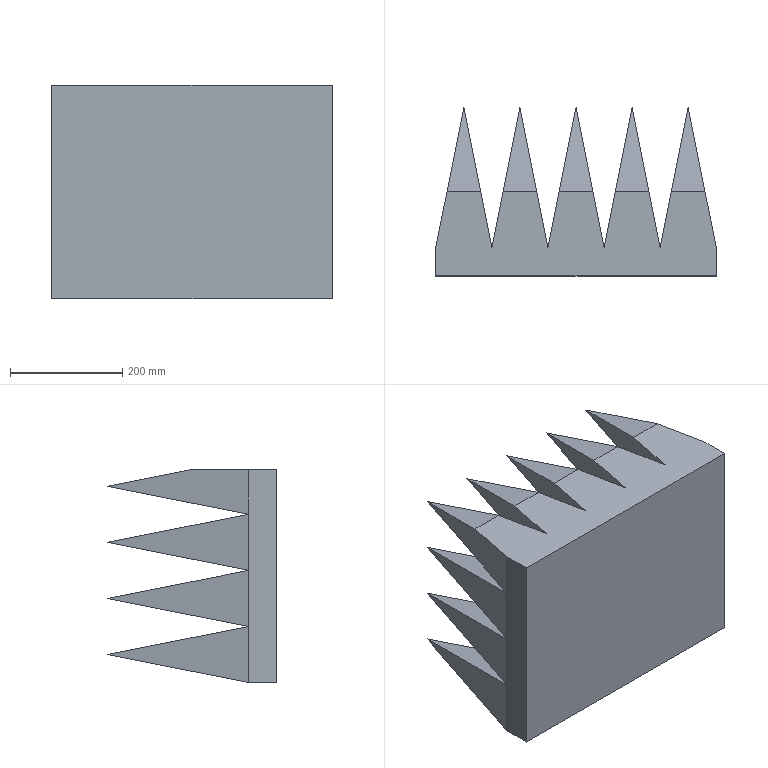Part | SolidWorks | features LPattern 2, Blend 1, Extrusion 1, ICE 1 | 1 solid | 85 faces | box 500 x 300 x 380 mm | volume 25733333 mm3 | plane 85